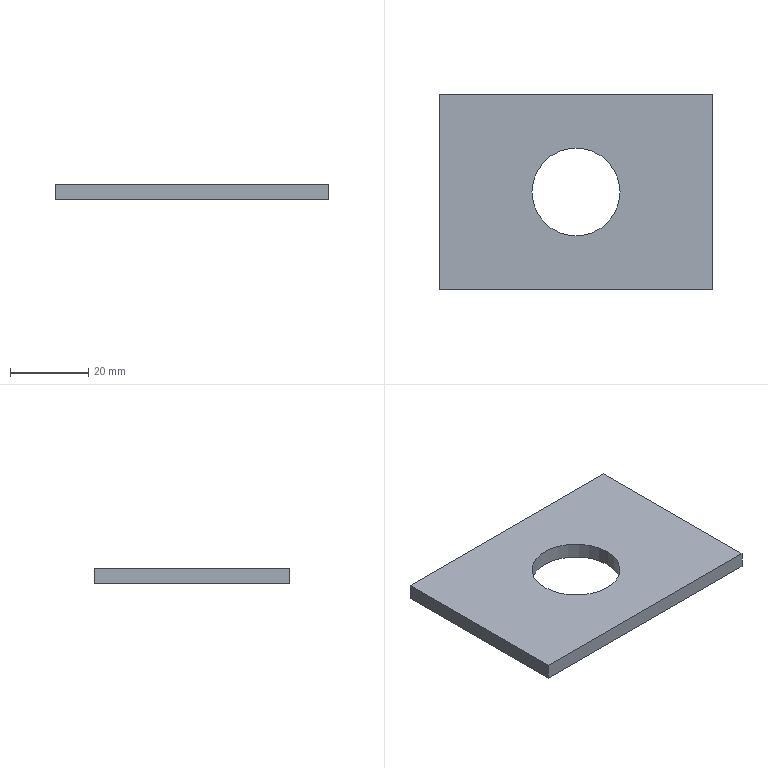Part | STEP file | 2012-06-08-08 | 1 solid | 8 faces | box 70 x 50 x 4 mm | volume 12410 mm3 | plane 6 | cylinder 2 | commonest cylinder face diameters 22.5 x2
STEP:
#1=CARTESIAN_POINT('',(0.,0.,0.));
#2=DIRECTION('',(0.,0.,1.));
#3=DIRECTION('',(1.,0.,0.));
#4=AXIS2_PLACEMENT_3D('',#1,#2,#3);
#5=CARTESIAN_POINT('',(-11.25,0.,4.));
#6=VERTEX_POINT('',#5);
#7=CARTESIAN_POINT('',(-11.25,0.,0.));
#8=VERTEX_POINT('',#7);
#9=CARTESIAN_POINT('',(-11.25,0.,4.));
#10=DIRECTION('',(0.,0.,-1.));
#11=VECTOR('',#10,1.);
#12=LINE('',#9,#11);
#13=CARTESIAN_POINT('',(0.,0.,4.));
#14=DIRECTION('',(0.,0.,-1.));
#15=DIRECTION('',(-1.,0.,0.));
#16=AXIS2_PLACEMENT_3D('',#13,#14,#15);
#17=CYLINDRICAL_SURFACE('',#16,11.25);
#18=CARTESIAN_POINT('',(6.283,0.));
#19=DIRECTION('',(0.,1.));
#20=VECTOR('',#19,1.);
#21=LINE('',#18,#20);
#22=(GEOMETRIC_REPRESENTATION_CONTEXT(2)PARAMETRIC_REPRESENTATION_CONTEXT()REPRESENTATION_CONTEXT('',''));
#23=DEFINITIONAL_REPRESENTATION('',(#21),#22);
#24=PCURVE('',#17,#23);
#25=CARTESIAN_POINT('',(0.,0.,4.));
#26=DIRECTION('',(0.,0.,-1.));
#27=DIRECTION('',(-1.,0.,0.));
#28=AXIS2_PLACEMENT_3D('',#25,#26,#27);
#29=CYLINDRICAL_SURFACE('',#28,11.25);
#30=CARTESIAN_POINT('',(0.,0.));
#31=DIRECTION('',(0.,1.));
#32=VECTOR('',#31,1.);
#33=LINE('',#30,#32);
#34=(GEOMETRIC_REPRESENTATION_CONTEXT(2)PARAMETRIC_REPRESENTATION_CONTEXT()REPRESENTATION_CONTEXT('',''));
#35=DEFINITIONAL_REPRESENTATION('',(#33),#34);
#36=PCURVE('',#29,#35);
#37=SURFACE_CURVE('',#12,(#24,#36),.PCURVE_S1.);
#38=EDGE_CURVE('',#6,#8,#37,.T.);
#39=ORIENTED_EDGE('',*,*,#38,.T.);
#40=CARTESIAN_POINT('',(11.25,0.,0.));
#41=VERTEX_POINT('',#40);
#42=CARTESIAN_POINT('',(0.,0.,0.));
#43=DIRECTION('',(0.,0.,1.));
#44=DIRECTION('',(1.,0.,0.));
#45=AXIS2_PLACEMENT_3D('',#42,#43,#44);
#46=CIRCLE('',#45,11.25);
#47=CARTESIAN_POINT('',(9.425,4.));
#48=DIRECTION('',(-1.,0.));
#49=VECTOR('',#48,1.);
#50=LINE('',#47,#49);
#51=(GEOMETRIC_REPRESENTATION_CONTEXT(2)PARAMETRIC_REPRESENTATION_CONTEXT()REPRESENTATION_CONTEXT('',''));
#52=DEFINITIONAL_REPRESENTATION('',(#50),#51);
#53=PCURVE('',#17,#52);
#54=CARTESIAN_POINT('',(35.,-25.,0.));
#55=DIRECTION('',(0.,0.,1.));
#56=DIRECTION('',(1.,0.,0.));
#57=AXIS2_PLACEMENT_3D('',#54,#55,#56);
#58=PLANE('',#57);
#59=CARTESIAN_POINT('',(-35.,25.));
#60=DIRECTION('',(1.,0.));
#61=AXIS2_PLACEMENT_2D('',#59,#60);
#62=CIRCLE('',#61,11.25);
#63=(GEOMETRIC_REPRESENTATION_CONTEXT(2)PARAMETRIC_REPRESENTATION_CONTEXT()REPRESENTATION_CONTEXT('',''));
#64=DEFINITIONAL_REPRESENTATION('',(#62),#63);
#65=PCURVE('',#58,#64);
#66=SURFACE_CURVE('',#46,(#53,#65),.PCURVE_S1.);
#67=EDGE_CURVE('',#8,#41,#66,.T.);
#68=ORIENTED_EDGE('',*,*,#67,.T.);
#69=CARTESIAN_POINT('',(11.25,0.,4.));
#70=VERTEX_POINT('',#69);
#71=CARTESIAN_POINT('',(11.25,0.,4.));
#72=DIRECTION('',(0.,0.,-1.));
#73=VECTOR('',#72,1.);
#74=LINE('',#71,#73);
#75=CARTESIAN_POINT('',(3.142,0.));
#76=DIRECTION('',(0.,1.));
#77=VECTOR('',#76,1.);
#78=LINE('',#75,#77);
#79=(GEOMETRIC_REPRESENTATION_CONTEXT(2)PARAMETRIC_REPRESENTATION_CONTEXT()REPRESENTATION_CONTEXT('',''));
#80=DEFINITIONAL_REPRESENTATION('',(#78),#79);
#81=PCURVE('',#17,#80);
#82=CARTESIAN_POINT('',(3.142,0.));
#83=DIRECTION('',(0.,1.));
#84=VECTOR('',#83,1.);
#85=LINE('',#82,#84);
#86=(GEOMETRIC_REPRESENTATION_CONTEXT(2)PARAMETRIC_REPRESENTATION_CONTEXT()REPRESENTATION_CONTEXT('',''));
#87=DEFINITIONAL_REPRESENTATION('',(#85),#86);
#88=PCURVE('',#29,#87);
#89=SURFACE_CURVE('',#74,(#81,#88),.PCURVE_S1.);
#90=EDGE_CURVE('',#70,#41,#89,.T.);
#91=ORIENTED_EDGE('',*,*,#90,.F.);
#92=CARTESIAN_POINT('',(0.,0.,4.));
#93=DIRECTION('',(0.,0.,1.));
#94=DIRECTION('',(1.,0.,0.));
#95=AXIS2_PLACEMENT_3D('',#92,#93,#94);
#96=CIRCLE('',#95,11.25);
#97=CARTESIAN_POINT('',(9.425,0.));
#98=DIRECTION('',(-1.,0.));
#99=VECTOR('',#98,1.);
#100=LINE('',#97,#99);
#101=(GEOMETRIC_REPRESENTATION_CONTEXT(2)PARAMETRIC_REPRESENTATION_CONTEXT()REPRESENTATION_CONTEXT('',''));
#102=DEFINITIONAL_REPRESENTATION('',(#100),#101);
#103=PCURVE('',#17,#102);
#104=CARTESIAN_POINT('',(35.,-25.,4.));
#105=DIRECTION('',(0.,0.,1.));
#106=DIRECTION('',(1.,0.,0.));
#107=AXIS2_PLACEMENT_3D('',#104,#105,#106);
#108=PLANE('',#107);
#109=CARTESIAN_POINT('',(-35.,25.));
#110=DIRECTION('',(1.,0.));
#111=AXIS2_PLACEMENT_2D('',#109,#110);
#112=CIRCLE('',#111,11.25);
#113=(GEOMETRIC_REPRESENTATION_CONTEXT(2)PARAMETRIC_REPRESENTATION_CONTEXT()REPRESENTATION_CONTEXT('',''));
#114=DEFINITIONAL_REPRESENTATION('',(#112),#113);
#115=PCURVE('',#108,#114);
#116=SURFACE_CURVE('',#96,(#103,#115),.PCURVE_S1.);
#117=EDGE_CURVE('',#6,#70,#116,.T.);
#118=ORIENTED_EDGE('',*,*,#117,.F.);
#119=EDGE_LOOP('',(#39,#68,#91,#118));
#120=FACE_BOUND('',#119,.F.);
#121=ADVANCED_FACE('',(#120),#17,.F.);
#122=CARTESIAN_POINT('',(35.,-25.,4.));
#123=VERTEX_POINT('',#122);
#124=CARTESIAN_POINT('',(35.,25.,4.));
#125=VERTEX_POINT('',#124);
#126=CARTESIAN_POINT('',(35.,25.,4.));
#127=DIRECTION('',(0.,1.,0.));
#128=VECTOR('',#127,1.);
#129=LINE('',#126,#128);
#130=CARTESIAN_POINT('',(0.,50.));
#131=DIRECTION('',(0.,1.));
#132=VECTOR('',#131,1.);
#133=LINE('',#130,#132);
#134=(GEOMETRIC_REPRESENTATION_CONTEXT(2)PARAMETRIC_REPRESENTATION_CONTEXT()REPRESENTATION_CONTEXT('',''));
#135=DEFINITIONAL_REPRESENTATION('',(#133),#134);
#136=PCURVE('',#108,#135);
#137=CARTESIAN_POINT('',(35.,25.,4.));
#138=DIRECTION('',(-1.,0.,0.));
#139=DIRECTION('',(0.,-1.,0.));
#140=AXIS2_PLACEMENT_3D('',#137,#138,#139);
#141=PLANE('',#140);
#142=CARTESIAN_POINT('',(0.,0.));
#143=DIRECTION('',(-1.,0.));
#144=VECTOR('',#143,1.);
#145=LINE('',#142,#144);
#146=(GEOMETRIC_REPRESENTATION_CONTEXT(2)PARAMETRIC_REPRESENTATION_CONTEXT()REPRESENTATION_CONTEXT('',''));
#147=DEFINITIONAL_REPRESENTATION('',(#145),#146);
#148=PCURVE('',#141,#147);
#149=SURFACE_CURVE('',#129,(#136,#148),.PCURVE_S1.);
#150=EDGE_CURVE('',#123,#125,#149,.T.);
#151=ORIENTED_EDGE('',*,*,#150,.T.);
#152=CARTESIAN_POINT('',(-35.,25.,4.));
#153=VERTEX_POINT('',#152);
#154=CARTESIAN_POINT('',(-35.,25.,4.));
#155=DIRECTION('',(-1.,0.,0.));
#156=VECTOR('',#155,1.);
#157=LINE('',#154,#156);
#158=CARTESIAN_POINT('',(-70.,50.));
#159=DIRECTION('',(-1.,0.));
#160=VECTOR('',#159,1.);
#161=LINE('',#158,#160);
#162=(GEOMETRIC_REPRESENTATION_CONTEXT(2)PARAMETRIC_REPRESENTATION_CONTEXT()REPRESENTATION_CONTEXT('',''));
#163=DEFINITIONAL_REPRESENTATION('',(#161),#162);
#164=PCURVE('',#108,#163);
#165=CARTESIAN_POINT('',(-35.,25.,4.));
#166=DIRECTION('',(0.,-1.,0.));
#167=DIRECTION('',(0.,0.,-1.));
#168=AXIS2_PLACEMENT_3D('',#165,#166,#167);
#169=PLANE('',#168);
#170=CARTESIAN_POINT('',(0.,0.));
#171=DIRECTION('',(0.,-1.));
#172=VECTOR('',#171,1.);
#173=LINE('',#170,#172);
#174=(GEOMETRIC_REPRESENTATION_CONTEXT(2)PARAMETRIC_REPRESENTATION_CONTEXT()REPRESENTATION_CONTEXT('',''));
#175=DEFINITIONAL_REPRESENTATION('',(#173),#174);
#176=PCURVE('',#169,#175);
#177=SURFACE_CURVE('',#157,(#164,#176),.PCURVE_S1.);
#178=EDGE_CURVE('',#125,#153,#177,.T.);
#179=ORIENTED_EDGE('',*,*,#178,.T.);
#180=CARTESIAN_POINT('',(-35.,-25.,4.));
#181=VERTEX_POINT('',#180);
#182=CARTESIAN_POINT('',(-35.,25.,4.));
#183=DIRECTION('',(0.,-1.,0.));
#184=VECTOR('',#183,1.);
#185=LINE('',#182,#184);
#186=CARTESIAN_POINT('',(-70.,50.));
#187=DIRECTION('',(0.,-1.));
#188=VECTOR('',#187,1.);
#189=LINE('',#186,#188);
#190=(GEOMETRIC_REPRESENTATION_CONTEXT(2)PARAMETRIC_REPRESENTATION_CONTEXT()REPRESENTATION_CONTEXT('',''));
#191=DEFINITIONAL_REPRESENTATION('',(#189),#190);
#192=PCURVE('',#108,#191);
#193=CARTESIAN_POINT('',(-35.,25.,4.));
#194=DIRECTION('',(1.,0.,0.));
#195=DIRECTION('',(0.,1.,0.));
#196=AXIS2_PLACEMENT_3D('',#193,#194,#195);
#197=PLANE('',#196);
#198=CARTESIAN_POINT('',(0.,0.));
#199=DIRECTION('',(-1.,0.));
#200=VECTOR('',#199,1.);
#201=LINE('',#198,#200);
#202=(GEOMETRIC_REPRESENTATION_CONTEXT(2)PARAMETRIC_REPRESENTATION_CONTEXT()REPRESENTATION_CONTEXT('',''));
#203=DEFINITIONAL_REPRESENTATION('',(#201),#202);
#204=PCURVE('',#197,#203);
#205=SURFACE_CURVE('',#185,(#192,#204),.PCURVE_S1.);
#206=EDGE_CURVE('',#153,#181,#205,.T.);
#207=ORIENTED_EDGE('',*,*,#206,.T.);
#208=CARTESIAN_POINT('',(-35.,-25.,4.));
#209=DIRECTION('',(1.,0.,0.));
#210=VECTOR('',#209,1.);
#211=LINE('',#208,#210);
#212=CARTESIAN_POINT('',(-70.,0.));
#213=DIRECTION('',(1.,0.));
#214=VECTOR('',#213,1.);
#215=LINE('',#212,#214);
#216=(GEOMETRIC_REPRESENTATION_CONTEXT(2)PARAMETRIC_REPRESENTATION_CONTEXT()REPRESENTATION_CONTEXT('',''));
#217=DEFINITIONAL_REPRESENTATION('',(#215),#216);
#218=PCURVE('',#108,#217);
#219=CARTESIAN_POINT('',(-35.,-25.,4.));
#220=DIRECTION('',(0.,1.,0.));
#221=DIRECTION('',(0.,0.,1.));
#222=AXIS2_PLACEMENT_3D('',#219,#220,#221);
#223=PLANE('',#222);
#224=CARTESIAN_POINT('',(0.,0.));
#225=DIRECTION('',(0.,1.));
#226=VECTOR('',#225,1.);
#227=LINE('',#224,#226);
#228=(GEOMETRIC_REPRESENTATION_CONTEXT(2)PARAMETRIC_REPRESENTATION_CONTEXT()REPRESENTATION_CONTEXT('',''));
#229=DEFINITIONAL_REPRESENTATION('',(#227),#228);
#230=PCURVE('',#223,#229);
#231=SURFACE_CURVE('',#211,(#218,#230),.PCURVE_S1.);
#232=EDGE_CURVE('',#181,#123,#231,.T.);
#233=ORIENTED_EDGE('',*,*,#232,.T.);
#234=EDGE_LOOP('',(#151,#179,#207,#233));
#235=FACE_BOUND('',#234,.T.);
#236=ORIENTED_EDGE('',*,*,#117,.F.);
#237=CARTESIAN_POINT('',(0.,0.,4.));
#238=DIRECTION('',(0.,0.,1.));
#239=DIRECTION('',(1.,0.,0.));
#240=AXIS2_PLACEMENT_3D('',#237,#238,#239);
#241=CIRCLE('',#240,11.25);
#242=CARTESIAN_POINT('',(-35.,25.));
#243=DIRECTION('',(1.,0.));
#244=AXIS2_PLACEMENT_2D('',#242,#243);
#245=CIRCLE('',#244,11.25);
#246=(GEOMETRIC_REPRESENTATION_CONTEXT(2)PARAMETRIC_REPRESENTATION_CONTEXT()REPRESENTATION_CONTEXT('',''));
#247=DEFINITIONAL_REPRESENTATION('',(#245),#246);
#248=PCURVE('',#108,#247);
#249=CARTESIAN_POINT('',(3.142,0.));
#250=DIRECTION('',(-1.,0.));
#251=VECTOR('',#250,1.);
#252=LINE('',#249,#251);
#253=(GEOMETRIC_REPRESENTATION_CONTEXT(2)PARAMETRIC_REPRESENTATION_CONTEXT()REPRESENTATION_CONTEXT('',''));
#254=DEFINITIONAL_REPRESENTATION('',(#252),#253);
#255=PCURVE('',#29,#254);
#256=SURFACE_CURVE('',#241,(#248,#255),.PCURVE_S1.);
#257=EDGE_CURVE('',#70,#6,#256,.T.);
#258=ORIENTED_EDGE('',*,*,#257,.F.);
#259=EDGE_LOOP('',(#236,#258));
#260=FACE_BOUND('',#259,.T.);
#261=ADVANCED_FACE('',(#235,#260),#108,.T.);
#262=CARTESIAN_POINT('',(35.,-25.,0.));
#263=VERTEX_POINT('',#262);
#264=CARTESIAN_POINT('',(35.,25.,0.));
#265=VERTEX_POINT('',#264);
#266=CARTESIAN_POINT('',(35.,25.,0.));
#267=DIRECTION('',(0.,1.,0.));
#268=VECTOR('',#267,1.);
#269=LINE('',#266,#268);
#270=CARTESIAN_POINT('',(0.,50.));
#271=DIRECTION('',(0.,1.));
#272=VECTOR('',#271,1.);
#273=LINE('',#270,#272);
#274=(GEOMETRIC_REPRESENTATION_CONTEXT(2)PARAMETRIC_REPRESENTATION_CONTEXT()REPRESENTATION_CONTEXT('',''));
#275=DEFINITIONAL_REPRESENTATION('',(#273),#274);
#276=PCURVE('',#58,#275);
#277=CARTESIAN_POINT('',(0.,-4.));
#278=DIRECTION('',(-1.,0.));
#279=VECTOR('',#278,1.);
#280=LINE('',#277,#279);
#281=(GEOMETRIC_REPRESENTATION_CONTEXT(2)PARAMETRIC_REPRESENTATION_CONTEXT()REPRESENTATION_CONTEXT('',''));
#282=DEFINITIONAL_REPRESENTATION('',(#280),#281);
#283=PCURVE('',#141,#282);
#284=SURFACE_CURVE('',#269,(#276,#283),.PCURVE_S1.);
#285=EDGE_CURVE('',#263,#265,#284,.T.);
#286=ORIENTED_EDGE('',*,*,#285,.F.);
#287=CARTESIAN_POINT('',(-35.,-25.,0.));
#288=VERTEX_POINT('',#287);
#289=CARTESIAN_POINT('',(-35.,-25.,0.));
#290=DIRECTION('',(1.,0.,0.));
#291=VECTOR('',#290,1.);
#292=LINE('',#289,#291);
#293=CARTESIAN_POINT('',(-70.,0.));
#294=DIRECTION('',(1.,0.));
#295=VECTOR('',#294,1.);
#296=LINE('',#293,#295);
#297=(GEOMETRIC_REPRESENTATION_CONTEXT(2)PARAMETRIC_REPRESENTATION_CONTEXT()REPRESENTATION_CONTEXT('',''));
#298=DEFINITIONAL_REPRESENTATION('',(#296),#297);
#299=PCURVE('',#58,#298);
#300=CARTESIAN_POINT('',(-4.,0.));
#301=DIRECTION('',(0.,1.));
#302=VECTOR('',#301,1.);
#303=LINE('',#300,#302);
#304=(GEOMETRIC_REPRESENTATION_CONTEXT(2)PARAMETRIC_REPRESENTATION_CONTEXT()REPRESENTATION_CONTEXT('',''));
#305=DEFINITIONAL_REPRESENTATION('',(#303),#304);
#306=PCURVE('',#223,#305);
#307=SURFACE_CURVE('',#292,(#299,#306),.PCURVE_S1.);
#308=EDGE_CURVE('',#288,#263,#307,.T.);
#309=ORIENTED_EDGE('',*,*,#308,.F.);
#310=CARTESIAN_POINT('',(-35.,25.,0.));
#311=VERTEX_POINT('',#310);
#312=CARTESIAN_POINT('',(-35.,25.,0.));
#313=DIRECTION('',(0.,-1.,0.));
#314=VECTOR('',#313,1.);
#315=LINE('',#312,#314);
#316=CARTESIAN_POINT('',(-70.,50.));
#317=DIRECTION('',(0.,-1.));
#318=VECTOR('',#317,1.);
#319=LINE('',#316,#318);
#320=(GEOMETRIC_REPRESENTATION_CONTEXT(2)PARAMETRIC_REPRESENTATION_CONTEXT()REPRESENTATION_CONTEXT('',''));
#321=DEFINITIONAL_REPRESENTATION('',(#319),#320);
#322=PCURVE('',#58,#321);
#323=CARTESIAN_POINT('',(0.,-4.));
#324=DIRECTION('',(-1.,0.));
#325=VECTOR('',#324,1.);
#326=LINE('',#323,#325);
#327=(GEOMETRIC_REPRESENTATION_CONTEXT(2)PARAMETRIC_REPRESENTATION_CONTEXT()REPRESENTATION_CONTEXT('',''));
#328=DEFINITIONAL_REPRESENTATION('',(#326),#327);
#329=PCURVE('',#197,#328);
#330=SURFACE_CURVE('',#315,(#322,#329),.PCURVE_S1.);
#331=EDGE_CURVE('',#311,#288,#330,.T.);
#332=ORIENTED_EDGE('',*,*,#331,.F.);
#333=CARTESIAN_POINT('',(-35.,25.,0.));
#334=DIRECTION('',(-1.,0.,0.));
#335=VECTOR('',#334,1.);
#336=LINE('',#333,#335);
#337=CARTESIAN_POINT('',(-70.,50.));
#338=DIRECTION('',(-1.,0.));
#339=VECTOR('',#338,1.);
#340=LINE('',#337,#339);
#341=(GEOMETRIC_REPRESENTATION_CONTEXT(2)PARAMETRIC_REPRESENTATION_CONTEXT()REPRESENTATION_CONTEXT('',''));
#342=DEFINITIONAL_REPRESENTATION('',(#340),#341);
#343=PCURVE('',#58,#342);
#344=CARTESIAN_POINT('',(4.,0.));
#345=DIRECTION('',(0.,-1.));
#346=VECTOR('',#345,1.);
#347=LINE('',#344,#346);
#348=(GEOMETRIC_REPRESENTATION_CONTEXT(2)PARAMETRIC_REPRESENTATION_CONTEXT()REPRESENTATION_CONTEXT('',''));
#349=DEFINITIONAL_REPRESENTATION('',(#347),#348);
#350=PCURVE('',#169,#349);
#351=SURFACE_CURVE('',#336,(#343,#350),.PCURVE_S1.);
#352=EDGE_CURVE('',#265,#311,#351,.T.);
#353=ORIENTED_EDGE('',*,*,#352,.F.);
#354=EDGE_LOOP('',(#286,#309,#332,#353));
#355=FACE_BOUND('',#354,.T.);
#356=ORIENTED_EDGE('',*,*,#67,.T.);
#357=CARTESIAN_POINT('',(0.,0.,0.));
#358=DIRECTION('',(0.,0.,1.));
#359=DIRECTION('',(1.,0.,0.));
#360=AXIS2_PLACEMENT_3D('',#357,#358,#359);
#361=CIRCLE('',#360,11.25);
#362=CARTESIAN_POINT('',(-35.,25.));
#363=DIRECTION('',(1.,0.));
#364=AXIS2_PLACEMENT_2D('',#362,#363);
#365=CIRCLE('',#364,11.25);
#366=(GEOMETRIC_REPRESENTATION_CONTEXT(2)PARAMETRIC_REPRESENTATION_CONTEXT()REPRESENTATION_CONTEXT('',''));
#367=DEFINITIONAL_REPRESENTATION('',(#365),#366);
#368=PCURVE('',#58,#367);
#369=CARTESIAN_POINT('',(3.142,4.));
#370=DIRECTION('',(-1.,0.));
#371=VECTOR('',#370,1.);
#372=LINE('',#369,#371);
#373=(GEOMETRIC_REPRESENTATION_CONTEXT(2)PARAMETRIC_REPRESENTATION_CONTEXT()REPRESENTATION_CONTEXT('',''));
#374=DEFINITIONAL_REPRESENTATION('',(#372),#373);
#375=PCURVE('',#29,#374);
#376=SURFACE_CURVE('',#361,(#368,#375),.PCURVE_S1.);
#377=EDGE_CURVE('',#41,#8,#376,.T.);
#378=ORIENTED_EDGE('',*,*,#377,.T.);
#379=EDGE_LOOP('',(#356,#378));
#380=FACE_BOUND('',#379,.T.);
#381=ADVANCED_FACE('',(#355,#380),#58,.F.);
#382=ORIENTED_EDGE('',*,*,#285,.T.);
#383=CARTESIAN_POINT('',(35.,25.,4.));
#384=DIRECTION('',(0.,0.,-1.));
#385=VECTOR('',#384,1.);
#386=LINE('',#383,#385);
#387=CARTESIAN_POINT('',(0.,0.));
#388=DIRECTION('',(0.,-1.));
#389=VECTOR('',#388,1.);
#390=LINE('',#387,#389);
#391=(GEOMETRIC_REPRESENTATION_CONTEXT(2)PARAMETRIC_REPRESENTATION_CONTEXT()REPRESENTATION_CONTEXT('',''));
#392=DEFINITIONAL_REPRESENTATION('',(#390),#391);
#393=PCURVE('',#141,#392);
#394=CARTESIAN_POINT('',(0.,70.));
#395=DIRECTION('',(1.,0.));
#396=VECTOR('',#395,1.);
#397=LINE('',#394,#396);
#398=(GEOMETRIC_REPRESENTATION_CONTEXT(2)PARAMETRIC_REPRESENTATION_CONTEXT()REPRESENTATION_CONTEXT('',''));
#399=DEFINITIONAL_REPRESENTATION('',(#397),#398);
#400=PCURVE('',#169,#399);
#401=SURFACE_CURVE('',#386,(#393,#400),.PCURVE_S1.);
#402=EDGE_CURVE('',#125,#265,#401,.T.);
#403=ORIENTED_EDGE('',*,*,#402,.F.);
#404=ORIENTED_EDGE('',*,*,#150,.F.);
#405=CARTESIAN_POINT('',(35.,-25.,4.));
#406=DIRECTION('',(0.,0.,-1.));
#407=VECTOR('',#406,1.);
#408=LINE('',#405,#407);
#409=CARTESIAN_POINT('',(50.,0.));
#410=DIRECTION('',(0.,-1.));
#411=VECTOR('',#410,1.);
#412=LINE('',#409,#411);
#413=(GEOMETRIC_REPRESENTATION_CONTEXT(2)PARAMETRIC_REPRESENTATION_CONTEXT()REPRESENTATION_CONTEXT('',''));
#414=DEFINITIONAL_REPRESENTATION('',(#412),#413);
#415=PCURVE('',#141,#414);
#416=CARTESIAN_POINT('',(0.,70.));
#417=DIRECTION('',(-1.,0.));
#418=VECTOR('',#417,1.);
#419=LINE('',#416,#418);
#420=(GEOMETRIC_REPRESENTATION_CONTEXT(2)PARAMETRIC_REPRESENTATION_CONTEXT()REPRESENTATION_CONTEXT('',''));
#421=DEFINITIONAL_REPRESENTATION('',(#419),#420);
#422=PCURVE('',#223,#421);
#423=SURFACE_CURVE('',#408,(#415,#422),.PCURVE_S1.);
#424=EDGE_CURVE('',#123,#263,#423,.T.);
#425=ORIENTED_EDGE('',*,*,#424,.T.);
#426=EDGE_LOOP('',(#382,#403,#404,#425));
#427=FACE_BOUND('',#426,.T.);
#428=ADVANCED_FACE('',(#427),#141,.F.);
#429=ORIENTED_EDGE('',*,*,#352,.T.);
#430=CARTESIAN_POINT('',(-35.,25.,4.));
#431=DIRECTION('',(0.,0.,-1.));
#432=VECTOR('',#431,1.);
#433=LINE('',#430,#432);
#434=CARTESIAN_POINT('',(0.,0.));
#435=DIRECTION('',(1.,0.));
#436=VECTOR('',#435,1.);
#437=LINE('',#434,#436);
#438=(GEOMETRIC_REPRESENTATION_CONTEXT(2)PARAMETRIC_REPRESENTATION_CONTEXT()REPRESENTATION_CONTEXT('',''));
#439=DEFINITIONAL_REPRESENTATION('',(#437),#438);
#440=PCURVE('',#169,#439);
#441=CARTESIAN_POINT('',(0.,0.));
#442=DIRECTION('',(0.,-1.));
#443=VECTOR('',#442,1.);
#444=LINE('',#441,#443);
#445=(GEOMETRIC_REPRESENTATION_CONTEXT(2)PARAMETRIC_REPRESENTATION_CONTEXT()REPRESENTATION_CONTEXT('',''));
#446=DEFINITIONAL_REPRESENTATION('',(#444),#445);
#447=PCURVE('',#197,#446);
#448=SURFACE_CURVE('',#433,(#440,#447),.PCURVE_S1.);
#449=EDGE_CURVE('',#153,#311,#448,.T.);
#450=ORIENTED_EDGE('',*,*,#449,.F.);
#451=ORIENTED_EDGE('',*,*,#178,.F.);
#452=ORIENTED_EDGE('',*,*,#402,.T.);
#453=EDGE_LOOP('',(#429,#450,#451,#452));
#454=FACE_BOUND('',#453,.T.);
#455=ADVANCED_FACE('',(#454),#169,.F.);
#456=ORIENTED_EDGE('',*,*,#331,.T.);
#457=CARTESIAN_POINT('',(-35.,-25.,4.));
#458=DIRECTION('',(0.,0.,-1.));
#459=VECTOR('',#458,1.);
#460=LINE('',#457,#459);
#461=CARTESIAN_POINT('',(-50.,0.));
#462=DIRECTION('',(0.,-1.));
#463=VECTOR('',#462,1.);
#464=LINE('',#461,#463);
#465=(GEOMETRIC_REPRESENTATION_CONTEXT(2)PARAMETRIC_REPRESENTATION_CONTEXT()REPRESENTATION_CONTEXT('',''));
#466=DEFINITIONAL_REPRESENTATION('',(#464),#465);
#467=PCURVE('',#197,#466);
#468=CARTESIAN_POINT('',(0.,0.));
#469=DIRECTION('',(-1.,0.));
#470=VECTOR('',#469,1.);
#471=LINE('',#468,#470);
#472=(GEOMETRIC_REPRESENTATION_CONTEXT(2)PARAMETRIC_REPRESENTATION_CONTEXT()REPRESENTATION_CONTEXT('',''));
#473=DEFINITIONAL_REPRESENTATION('',(#471),#472);
#474=PCURVE('',#223,#473);
#475=SURFACE_CURVE('',#460,(#467,#474),.PCURVE_S1.);
#476=EDGE_CURVE('',#181,#288,#475,.T.);
#477=ORIENTED_EDGE('',*,*,#476,.F.);
#478=ORIENTED_EDGE('',*,*,#206,.F.);
#479=ORIENTED_EDGE('',*,*,#449,.T.);
#480=EDGE_LOOP('',(#456,#477,#478,#479));
#481=FACE_BOUND('',#480,.T.);
#482=ADVANCED_FACE('',(#481),#197,.F.);
#483=ORIENTED_EDGE('',*,*,#308,.T.);
#484=ORIENTED_EDGE('',*,*,#424,.F.);
#485=ORIENTED_EDGE('',*,*,#232,.F.);
#486=ORIENTED_EDGE('',*,*,#476,.T.);
#487=EDGE_LOOP('',(#483,#484,#485,#486));
#488=FACE_BOUND('',#487,.T.);
#489=ADVANCED_FACE('',(#488),#223,.F.);
#490=ORIENTED_EDGE('',*,*,#377,.T.);
#491=ORIENTED_EDGE('',*,*,#38,.F.);
#492=ORIENTED_EDGE('',*,*,#257,.F.);
#493=ORIENTED_EDGE('',*,*,#90,.T.);
#494=EDGE_LOOP('',(#490,#491,#492,#493));
#495=FACE_BOUND('',#494,.F.);
#496=ADVANCED_FACE('',(#495),#29,.F.);
#497=CLOSED_SHELL('',(#121,#261,#381,#428,#455,#482,#489,#496));
#498=MANIFOLD_SOLID_BREP('',#497);
#499=(LENGTH_UNIT()NAMED_UNIT(*)SI_UNIT(.MILLI.,.METRE.));
#500=UNCERTAINTY_MEASURE_WITH_UNIT(LENGTH_MEASURE(0.0000001),#499,'','');
#501=(NAMED_UNIT(*)PLANE_ANGLE_UNIT()SI_UNIT($,.RADIAN.));
#502=(NAMED_UNIT(*)SI_UNIT($,.STERADIAN.)SOLID_ANGLE_UNIT());
#503=(GEOMETRIC_REPRESENTATION_CONTEXT(3)GLOBAL_UNCERTAINTY_ASSIGNED_CONTEXT((#500))GLOBAL_UNIT_ASSIGNED_CONTEXT((#499,#501,#502))REPRESENTATION_CONTEXT('',''));
#504=ADVANCED_BREP_SHAPE_REPRESENTATION('',(#4,#498),#503);